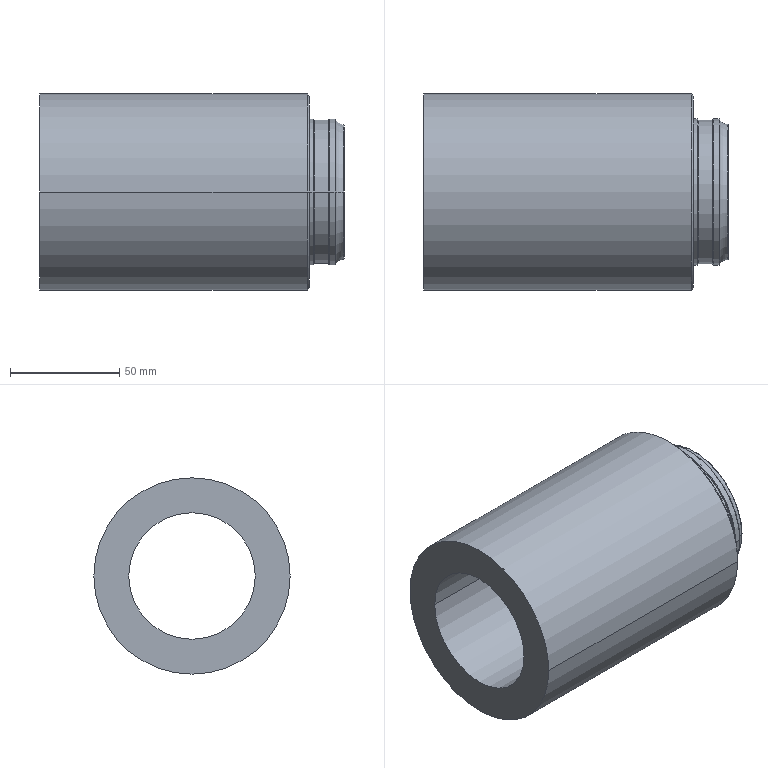Part | SolidWorks | features Revolution 1 | 1 solid | 31 faces | box 139.56 x 90 x 90 mm | volume 471413 mm3 | torus 14 | cylinder 10 | plane 5 | cone 2 | commonest cylinder face diameters 67 x4 58 x2 66 x2 90 x2
STEP:
#1=CARTESIAN_POINT('',(441.026,-31.014,0.));
#2=VERTEX_POINT('',#1);
#3=CARTESIAN_POINT('',(441.026,31.014,0.));
#4=VERTEX_POINT('',#3);
#5=CARTESIAN_POINT('',(441.026,0.,0.));
#6=DIRECTION('',(1.,0.,0.));
#7=DIRECTION('',(0.,1.,0.));
#8=AXIS2_PLACEMENT_3D('',#5,#6,#7);
#9=CIRCLE('',#8,31.014);
#10=EDGE_CURVE('',#2,#4,#9,.T.);
#11=ORIENTED_EDGE('',*,*,#10,.F.);
#12=CARTESIAN_POINT('',(437.44,-33.396,0.));
#13=VERTEX_POINT('',#12);
#14=CARTESIAN_POINT('',(441.503,-35.622,0.));
#15=DIRECTION('',(0.,0.,1.));
#16=DIRECTION('',(0.,-1.,0.));
#17=AXIS2_PLACEMENT_3D('',#14,#15,#16);
#18=CIRCLE('',#17,4.633);
#19=EDGE_CURVE('',#2,#13,#18,.T.);
#20=ORIENTED_EDGE('',*,*,#19,.T.);
#21=CARTESIAN_POINT('',(437.44,33.396,0.));
#22=VERTEX_POINT('',#21);
#23=CARTESIAN_POINT('',(437.44,0.,0.));
#24=DIRECTION('',(1.,0.,0.));
#25=DIRECTION('',(0.,1.,0.));
#26=AXIS2_PLACEMENT_3D('',#23,#24,#25);
#27=CIRCLE('',#26,33.396);
#28=EDGE_CURVE('',#13,#22,#27,.T.);
#29=ORIENTED_EDGE('',*,*,#28,.T.);
#30=CARTESIAN_POINT('',(441.503,35.622,0.));
#31=DIRECTION('',(0.,0.,-1.));
#32=DIRECTION('',(-1.,0.,0.));
#33=AXIS2_PLACEMENT_3D('',#30,#31,#32);
#34=CIRCLE('',#33,4.633);
#35=EDGE_CURVE('',#4,#22,#34,.T.);
#36=ORIENTED_EDGE('',*,*,#35,.F.);
#37=EDGE_LOOP('',(#11,#20,#29,#36));
#38=FACE_OUTER_BOUND('',#37,.T.);
#39=CARTESIAN_POINT('',(441.503,0.,0.));
#40=DIRECTION('',(1.,0.,0.));
#41=DIRECTION('',(0.,1.,0.));
#42=AXIS2_PLACEMENT_3D('',#39,#40,#41);
#43=TOROIDAL_SURFACE('',#42,35.622,4.633);
#44=ADVANCED_FACE('',(#38),#43,.F.);
#45=CARTESIAN_POINT('',(441.026,0.,0.));
#46=DIRECTION('',(1.,0.,0.));
#47=DIRECTION('',(0.,1.,0.));
#48=AXIS2_PLACEMENT_3D('',#45,#46,#47);
#49=CIRCLE('',#48,31.014);
#50=EDGE_CURVE('',#4,#2,#49,.T.);
#51=ORIENTED_EDGE('',*,*,#50,.T.);
#52=CARTESIAN_POINT('',(441.384,-30.616,0.));
#53=VERTEX_POINT('',#52);
#54=CARTESIAN_POINT('',(440.984,-30.616,0.));
#55=DIRECTION('',(0.,0.,1.));
#56=DIRECTION('',(0.,-1.,0.));
#57=AXIS2_PLACEMENT_3D('',#54,#55,#56);
#58=CIRCLE('',#57,0.4);
#59=EDGE_CURVE('',#2,#53,#58,.T.);
#60=ORIENTED_EDGE('',*,*,#59,.T.);
#61=CARTESIAN_POINT('',(441.384,30.616,0.));
#62=VERTEX_POINT('',#61);
#63=CARTESIAN_POINT('',(441.384,0.,0.));
#64=DIRECTION('',(1.,0.,0.));
#65=DIRECTION('',(0.,1.,0.));
#66=AXIS2_PLACEMENT_3D('',#63,#64,#65);
#67=CIRCLE('',#66,30.616);
#68=EDGE_CURVE('',#62,#53,#67,.T.);
#69=ORIENTED_EDGE('',*,*,#68,.F.);
#70=CARTESIAN_POINT('',(440.984,30.616,0.));
#71=DIRECTION('',(0.,0.,-1.));
#72=DIRECTION('',(-1.,0.,0.));
#73=AXIS2_PLACEMENT_3D('',#70,#71,#72);
#74=CIRCLE('',#73,0.4);
#75=EDGE_CURVE('',#4,#62,#74,.T.);
#76=ORIENTED_EDGE('',*,*,#75,.F.);
#77=EDGE_LOOP('',(#51,#60,#69,#76));
#78=FACE_OUTER_BOUND('',#77,.T.);
#79=CARTESIAN_POINT('',(440.984,0.,0.));
#80=DIRECTION('',(1.,0.,0.));
#81=DIRECTION('',(0.,1.,0.));
#82=AXIS2_PLACEMENT_3D('',#79,#80,#81);
#83=TOROIDAL_SURFACE('',#82,30.616,0.4);
#84=ADVANCED_FACE('',(#78),#83,.T.);
#85=CARTESIAN_POINT('',(301.824,-29.,0.));
#86=VERTEX_POINT('',#85);
#87=CARTESIAN_POINT('',(301.824,29.,0.));
#88=VERTEX_POINT('',#87);
#89=CARTESIAN_POINT('',(301.824,0.,0.));
#90=DIRECTION('',(1.,0.,0.));
#91=DIRECTION('',(0.,1.,0.));
#92=AXIS2_PLACEMENT_3D('',#89,#90,#91);
#93=CIRCLE('',#92,29.);
#94=EDGE_CURVE('',#86,#88,#93,.T.);
#95=ORIENTED_EDGE('',*,*,#94,.F.);
#96=CARTESIAN_POINT('',(441.384,-29.,0.));
#97=VERTEX_POINT('',#96);
#98=CARTESIAN_POINT('',(597.174,-29.,0.));
#99=DIRECTION('',(1.,0.,0.));
#100=VECTOR('',#99,1000.);
#101=LINE('',#98,#100);
#102=EDGE_CURVE('',#86,#97,#101,.T.);
#103=ORIENTED_EDGE('',*,*,#102,.T.);
#104=CARTESIAN_POINT('',(441.384,29.,0.));
#105=VERTEX_POINT('',#104);
#106=CARTESIAN_POINT('',(441.384,0.,0.));
#107=DIRECTION('',(1.,0.,0.));
#108=DIRECTION('',(0.,1.,0.));
#109=AXIS2_PLACEMENT_3D('',#106,#107,#108);
#110=CIRCLE('',#109,29.);
#111=EDGE_CURVE('',#97,#105,#110,.T.);
#112=ORIENTED_EDGE('',*,*,#111,.T.);
#113=CARTESIAN_POINT('',(597.174,29.,0.));
#114=DIRECTION('',(1.,0.,0.));
#115=VECTOR('',#114,1000.);
#116=LINE('',#113,#115);
#117=EDGE_CURVE('',#88,#105,#116,.T.);
#118=ORIENTED_EDGE('',*,*,#117,.F.);
#119=EDGE_LOOP('',(#95,#103,#112,#118));
#120=FACE_OUTER_BOUND('',#119,.T.);
#121=CARTESIAN_POINT('',(597.174,0.,0.));
#122=DIRECTION('',(1.,0.,0.));
#123=DIRECTION('',(0.,1.,0.));
#124=AXIS2_PLACEMENT_3D('',#121,#122,#123);
#125=CYLINDRICAL_SURFACE('',#124,29.);
#126=ADVANCED_FACE('',(#120),#125,.F.);
#127=CARTESIAN_POINT('',(301.824,45.,0.));
#128=VERTEX_POINT('',#127);
#129=CARTESIAN_POINT('',(301.824,-45.,0.));
#130=VERTEX_POINT('',#129);
#131=CARTESIAN_POINT('',(301.824,0.,0.));
#132=DIRECTION('',(1.,0.,0.));
#133=DIRECTION('',(0.,1.,0.));
#134=AXIS2_PLACEMENT_3D('',#131,#132,#133);
#135=CIRCLE('',#134,45.);
#136=EDGE_CURVE('',#128,#130,#135,.T.);
#137=ORIENTED_EDGE('',*,*,#136,.T.);
#138=CARTESIAN_POINT('',(424.384,-45.,0.));
#139=VERTEX_POINT('',#138);
#140=CARTESIAN_POINT('',(597.174,-45.,0.));
#141=DIRECTION('',(1.,0.,0.));
#142=VECTOR('',#141,1000.);
#143=LINE('',#140,#142);
#144=EDGE_CURVE('',#130,#139,#143,.T.);
#145=ORIENTED_EDGE('',*,*,#144,.T.);
#146=CARTESIAN_POINT('',(424.384,45.,0.));
#147=VERTEX_POINT('',#146);
#148=CARTESIAN_POINT('',(424.384,0.,0.));
#149=DIRECTION('',(1.,0.,0.));
#150=DIRECTION('',(0.,1.,0.));
#151=AXIS2_PLACEMENT_3D('',#148,#149,#150);
#152=CIRCLE('',#151,45.);
#153=EDGE_CURVE('',#147,#139,#152,.T.);
#154=ORIENTED_EDGE('',*,*,#153,.F.);
#155=CARTESIAN_POINT('',(597.174,45.,0.));
#156=DIRECTION('',(1.,0.,0.));
#157=VECTOR('',#156,1000.);
#158=LINE('',#155,#157);
#159=EDGE_CURVE('',#128,#147,#158,.T.);
#160=ORIENTED_EDGE('',*,*,#159,.F.);
#161=EDGE_LOOP('',(#137,#145,#154,#160));
#162=FACE_OUTER_BOUND('',#161,.T.);
#163=CARTESIAN_POINT('',(597.174,0.,0.));
#164=DIRECTION('',(1.,0.,0.));
#165=DIRECTION('',(0.,1.,0.));
#166=AXIS2_PLACEMENT_3D('',#163,#164,#165);
#167=CYLINDRICAL_SURFACE('',#166,45.);
#168=ADVANCED_FACE('',(#162),#167,.T.);
#169=CARTESIAN_POINT('',(425.384,44.,0.));
#170=VERTEX_POINT('',#169);
#171=CARTESIAN_POINT('',(425.384,-44.,0.));
#172=VERTEX_POINT('',#171);
#173=CARTESIAN_POINT('',(425.384,0.,0.));
#174=DIRECTION('',(1.,0.,0.));
#175=DIRECTION('',(0.,1.,0.));
#176=AXIS2_PLACEMENT_3D('',#173,#174,#175);
#177=CIRCLE('',#176,44.);
#178=EDGE_CURVE('',#170,#172,#177,.T.);
#179=ORIENTED_EDGE('',*,*,#178,.F.);
#180=CARTESIAN_POINT('',(425.384,44.,0.));
#181=DIRECTION('',(-0.7071,0.7071,0.));
#182=VECTOR('',#181,1000.);
#183=LINE('',#180,#182);
#184=EDGE_CURVE('',#170,#147,#183,.T.);
#185=ORIENTED_EDGE('',*,*,#184,.T.);
#186=ORIENTED_EDGE('',*,*,#153,.T.);
#187=CARTESIAN_POINT('',(425.384,-44.,0.));
#188=DIRECTION('',(-0.7071,-0.7071,0.));
#189=VECTOR('',#188,1000.);
#190=LINE('',#187,#189);
#191=EDGE_CURVE('',#172,#139,#190,.T.);
#192=ORIENTED_EDGE('',*,*,#191,.F.);
#193=EDGE_LOOP('',(#179,#185,#186,#192));
#194=FACE_OUTER_BOUND('',#193,.T.);
#195=CARTESIAN_POINT('',(425.384,0.,0.));
#196=DIRECTION('',(-1.,0.,0.));
#197=DIRECTION('',(0.,-1.,0.));
#198=AXIS2_PLACEMENT_3D('',#195,#196,#197);
#199=CONICAL_SURFACE('',#198,44.,0.7854);
#200=ADVANCED_FACE('',(#194),#199,.T.);
#201=CARTESIAN_POINT('',(425.384,33.5,0.));
#202=VERTEX_POINT('',#201);
#203=CARTESIAN_POINT('',(425.384,-33.5,0.));
#204=VERTEX_POINT('',#203);
#205=CARTESIAN_POINT('',(425.384,0.,0.));
#206=DIRECTION('',(1.,0.,0.));
#207=DIRECTION('',(0.,1.,0.));
#208=AXIS2_PLACEMENT_3D('',#205,#206,#207);
#209=CIRCLE('',#208,33.5);
#210=EDGE_CURVE('',#202,#204,#209,.T.);
#211=ORIENTED_EDGE('',*,*,#210,.T.);
#212=CARTESIAN_POINT('',(427.184,-33.5,0.));
#213=VERTEX_POINT('',#212);
#214=CARTESIAN_POINT('',(597.174,-33.5,0.));
#215=DIRECTION('',(1.,0.,0.));
#216=VECTOR('',#215,1000.);
#217=LINE('',#214,#216);
#218=EDGE_CURVE('',#204,#213,#217,.T.);
#219=ORIENTED_EDGE('',*,*,#218,.T.);
#220=CARTESIAN_POINT('',(427.184,33.5,0.));
#221=VERTEX_POINT('',#220);
#222=CARTESIAN_POINT('',(427.184,0.,0.));
#223=DIRECTION('',(1.,0.,0.));
#224=DIRECTION('',(0.,1.,0.));
#225=AXIS2_PLACEMENT_3D('',#222,#223,#224);
#226=CIRCLE('',#225,33.5);
#227=EDGE_CURVE('',#221,#213,#226,.T.);
#228=ORIENTED_EDGE('',*,*,#227,.F.);
#229=CARTESIAN_POINT('',(597.174,33.5,0.));
#230=DIRECTION('',(1.,0.,0.));
#231=VECTOR('',#230,1000.);
#232=LINE('',#229,#231);
#233=EDGE_CURVE('',#202,#221,#232,.T.);
#234=ORIENTED_EDGE('',*,*,#233,.F.);
#235=EDGE_LOOP('',(#211,#219,#228,#234));
#236=FACE_OUTER_BOUND('',#235,.T.);
#237=CARTESIAN_POINT('',(597.174,0.,0.));
#238=DIRECTION('',(1.,0.,0.));
#239=DIRECTION('',(0.,1.,0.));
#240=AXIS2_PLACEMENT_3D('',#237,#238,#239);
#241=CYLINDRICAL_SURFACE('',#240,33.5);
#242=ADVANCED_FACE('',(#236),#241,.T.);
#243=ORIENTED_EDGE('',*,*,#227,.T.);
#244=CARTESIAN_POINT('',(427.384,-33.3,0.));
#245=VERTEX_POINT('',#244);
#246=CARTESIAN_POINT('',(427.184,-33.3,0.));
#247=DIRECTION('',(0.,0.,1.));
#248=DIRECTION('',(0.,-1.,0.));
#249=AXIS2_PLACEMENT_3D('',#246,#247,#248);
#250=CIRCLE('',#249,0.2);
#251=EDGE_CURVE('',#213,#245,#250,.T.);
#252=ORIENTED_EDGE('',*,*,#251,.T.);
#253=CARTESIAN_POINT('',(427.384,33.3,0.));
#254=VERTEX_POINT('',#253);
#255=CARTESIAN_POINT('',(427.384,0.,0.));
#256=DIRECTION('',(1.,0.,0.));
#257=DIRECTION('',(0.,1.,0.));
#258=AXIS2_PLACEMENT_3D('',#255,#256,#257);
#259=CIRCLE('',#258,33.3);
#260=EDGE_CURVE('',#254,#245,#259,.T.);
#261=ORIENTED_EDGE('',*,*,#260,.F.);
#262=CARTESIAN_POINT('',(427.184,33.3,0.));
#263=DIRECTION('',(0.,0.,-1.));
#264=DIRECTION('',(-1.,0.,0.));
#265=AXIS2_PLACEMENT_3D('',#262,#263,#264);
#266=CIRCLE('',#265,0.2);
#267=EDGE_CURVE('',#221,#254,#266,.T.);
#268=ORIENTED_EDGE('',*,*,#267,.F.);
#269=EDGE_LOOP('',(#243,#252,#261,#268));
#270=FACE_OUTER_BOUND('',#269,.T.);
#271=CARTESIAN_POINT('',(427.184,0.,0.));
#272=DIRECTION('',(1.,0.,0.));
#273=DIRECTION('',(0.,1.,0.));
#274=AXIS2_PLACEMENT_3D('',#271,#272,#273);
#275=TOROIDAL_SURFACE('',#274,33.3,0.2);
#276=ADVANCED_FACE('',(#270),#275,.T.);
#277=CARTESIAN_POINT('',(427.584,-33.,0.));
#278=VERTEX_POINT('',#277);
#279=CARTESIAN_POINT('',(427.584,33.,0.));
#280=VERTEX_POINT('',#279);
#281=CARTESIAN_POINT('',(427.584,0.,0.));
#282=DIRECTION('',(1.,0.,0.));
#283=DIRECTION('',(0.,1.,0.));
#284=AXIS2_PLACEMENT_3D('',#281,#282,#283);
#285=CIRCLE('',#284,33.);
#286=EDGE_CURVE('',#278,#280,#285,.T.);
#287=ORIENTED_EDGE('',*,*,#286,.F.);
#288=CARTESIAN_POINT('',(427.384,-33.2,0.));
#289=VERTEX_POINT('',#288);
#290=CARTESIAN_POINT('',(427.584,-33.2,0.));
#291=DIRECTION('',(0.,0.,1.));
#292=DIRECTION('',(0.,-1.,0.));
#293=AXIS2_PLACEMENT_3D('',#290,#291,#292);
#294=CIRCLE('',#293,0.2);
#295=EDGE_CURVE('',#278,#289,#294,.T.);
#296=ORIENTED_EDGE('',*,*,#295,.T.);
#297=CARTESIAN_POINT('',(427.384,33.2,0.));
#298=VERTEX_POINT('',#297);
#299=CARTESIAN_POINT('',(427.384,0.,0.));
#300=DIRECTION('',(1.,0.,0.));
#301=DIRECTION('',(0.,1.,0.));
#302=AXIS2_PLACEMENT_3D('',#299,#300,#301);
#303=CIRCLE('',#302,33.2);
#304=EDGE_CURVE('',#289,#298,#303,.T.);
#305=ORIENTED_EDGE('',*,*,#304,.T.);
#306=CARTESIAN_POINT('',(427.584,33.2,0.));
#307=DIRECTION('',(0.,0.,-1.));
#308=DIRECTION('',(-1.,0.,0.));
#309=AXIS2_PLACEMENT_3D('',#306,#307,#308);
#310=CIRCLE('',#309,0.2);
#311=EDGE_CURVE('',#280,#298,#310,.T.);
#312=ORIENTED_EDGE('',*,*,#311,.F.);
#313=EDGE_LOOP('',(#287,#296,#305,#312));
#314=FACE_OUTER_BOUND('',#313,.T.);
#315=CARTESIAN_POINT('',(427.584,0.,0.));
#316=DIRECTION('',(1.,0.,0.));
#317=DIRECTION('',(0.,1.,0.));
#318=AXIS2_PLACEMENT_3D('',#315,#316,#317);
#319=TOROIDAL_SURFACE('',#318,33.2,0.2);
#320=ADVANCED_FACE('',(#314),#319,.F.);
#321=CARTESIAN_POINT('',(427.584,0.,0.));
#322=DIRECTION('',(1.,0.,0.));
#323=DIRECTION('',(0.,1.,0.));
#324=AXIS2_PLACEMENT_3D('',#321,#322,#323);
#325=CIRCLE('',#324,33.);
#326=EDGE_CURVE('',#280,#278,#325,.T.);
#327=ORIENTED_EDGE('',*,*,#326,.T.);
#328=CARTESIAN_POINT('',(434.184,-33.,0.));
#329=VERTEX_POINT('',#328);
#330=CARTESIAN_POINT('',(597.174,-33.,0.));
#331=DIRECTION('',(1.,0.,0.));
#332=VECTOR('',#331,1000.);
#333=LINE('',#330,#332);
#334=EDGE_CURVE('',#278,#329,#333,.T.);
#335=ORIENTED_EDGE('',*,*,#334,.T.);
#336=CARTESIAN_POINT('',(434.184,33.,0.));
#337=VERTEX_POINT('',#336);
#338=CARTESIAN_POINT('',(434.184,0.,0.));
#339=DIRECTION('',(1.,0.,0.));
#340=DIRECTION('',(0.,1.,0.));
#341=AXIS2_PLACEMENT_3D('',#338,#339,#340);
#342=CIRCLE('',#341,33.);
#343=EDGE_CURVE('',#337,#329,#342,.T.);
#344=ORIENTED_EDGE('',*,*,#343,.F.);
#345=CARTESIAN_POINT('',(597.174,33.,0.));
#346=DIRECTION('',(1.,0.,0.));
#347=VECTOR('',#346,1000.);
#348=LINE('',#345,#347);
#349=EDGE_CURVE('',#280,#337,#348,.T.);
#350=ORIENTED_EDGE('',*,*,#349,.F.);
#351=EDGE_LOOP('',(#327,#335,#344,#350));
#352=FACE_OUTER_BOUND('',#351,.T.);
#353=CARTESIAN_POINT('',(597.174,0.,0.));
#354=DIRECTION('',(1.,0.,0.));
#355=DIRECTION('',(0.,1.,0.));
#356=AXIS2_PLACEMENT_3D('',#353,#354,#355);
#357=CYLINDRICAL_SURFACE('',#356,33.);
#358=ADVANCED_FACE('',(#352),#357,.T.);
#359=CARTESIAN_POINT('',(434.384,-33.2,0.));
#360=VERTEX_POINT('',#359);
#361=CARTESIAN_POINT('',(434.384,33.2,0.));
#362=VERTEX_POINT('',#361);
#363=CARTESIAN_POINT('',(434.384,0.,0.));
#364=DIRECTION('',(1.,0.,0.));
#365=DIRECTION('',(0.,1.,0.));
#366=AXIS2_PLACEMENT_3D('',#363,#364,#365);
#367=CIRCLE('',#366,33.2);
#368=EDGE_CURVE('',#360,#362,#367,.T.);
#369=ORIENTED_EDGE('',*,*,#368,.F.);
#370=CARTESIAN_POINT('',(434.184,-33.2,0.));
#371=DIRECTION('',(0.,0.,1.));
#372=DIRECTION('',(0.,-1.,0.));
#373=AXIS2_PLACEMENT_3D('',#370,#371,#372);
#374=CIRCLE('',#373,0.2);
#375=EDGE_CURVE('',#360,#329,#374,.T.);
#376=ORIENTED_EDGE('',*,*,#375,.T.);
#377=CARTESIAN_POINT('',(434.184,0.,0.));
#378=DIRECTION('',(1.,0.,0.));
#379=DIRECTION('',(0.,1.,0.));
#380=AXIS2_PLACEMENT_3D('',#377,#378,#379);
#381=CIRCLE('',#380,33.);
#382=EDGE_CURVE('',#329,#337,#381,.T.);
#383=ORIENTED_EDGE('',*,*,#382,.T.);
#384=CARTESIAN_POINT('',(434.184,33.2,0.));
#385=DIRECTION('',(0.,0.,-1.));
#386=DIRECTION('',(-1.,0.,0.));
#387=AXIS2_PLACEMENT_3D('',#384,#385,#386);
#388=CIRCLE('',#387,0.2);
#389=EDGE_CURVE('',#362,#337,#388,.T.);
#390=ORIENTED_EDGE('',*,*,#389,.F.);
#391=EDGE_LOOP('',(#369,#376,#383,#390));
#392=FACE_OUTER_BOUND('',#391,.T.);
#393=CARTESIAN_POINT('',(434.184,0.,0.));
#394=DIRECTION('',(1.,0.,0.));
#395=DIRECTION('',(0.,1.,0.));
#396=AXIS2_PLACEMENT_3D('',#393,#394,#395);
#397=TOROIDAL_SURFACE('',#396,33.2,0.2);
#398=ADVANCED_FACE('',(#392),#397,.F.);
#399=CARTESIAN_POINT('',(434.384,33.3,0.));
#400=VERTEX_POINT('',#399);
#401=CARTESIAN_POINT('',(434.384,-33.3,0.));
#402=VERTEX_POINT('',#401);
#403=CARTESIAN_POINT('',(434.384,0.,0.));
#404=DIRECTION('',(1.,0.,0.));
#405=DIRECTION('',(0.,1.,0.));
#406=AXIS2_PLACEMENT_3D('',#403,#404,#405);
#407=CIRCLE('',#406,33.3);
#408=EDGE_CURVE('',#400,#402,#407,.T.);
#409=ORIENTED_EDGE('',*,*,#408,.T.);
#410=CARTESIAN_POINT('',(434.584,-33.5,0.));
#411=VERTEX_POINT('',#410);
#412=CARTESIAN_POINT('',(434.584,-33.3,0.));
#413=DIRECTION('',(0.,0.,1.));
#414=DIRECTION('',(0.,-1.,0.));
#415=AXIS2_PLACEMENT_3D('',#412,#413,#414);
#416=CIRCLE('',#415,0.2);
#417=EDGE_CURVE('',#402,#411,#416,.T.);
#418=ORIENTED_EDGE('',*,*,#417,.T.);
#419=CARTESIAN_POINT('',(434.584,33.5,0.));
#420=VERTEX_POINT('',#419);
#421=CARTESIAN_POINT('',(434.584,0.,0.));
#422=DIRECTION('',(1.,0.,0.));
#423=DIRECTION('',(0.,1.,0.));
#424=AXIS2_PLACEMENT_3D('',#421,#422,#423);
#425=CIRCLE('',#424,33.5);
#426=EDGE_CURVE('',#420,#411,#425,.T.);
#427=ORIENTED_EDGE('',*,*,#426,.F.);
#428=CARTESIAN_POINT('',(434.584,33.3,0.));
#429=DIRECTION('',(0.,0.,-1.));
#430=DIRECTION('',(-1.,0.,0.));
#431=AXIS2_PLACEMENT_3D('',#428,#429,#430);
#432=CIRCLE('',#431,0.2);
#433=EDGE_CURVE('',#400,#420,#432,.T.);
#434=ORIENTED_EDGE('',*,*,#433,.F.);
#435=EDGE_LOOP('',(#409,#418,#427,#434));
#436=FACE_OUTER_BOUND('',#435,.T.);
#437=CARTESIAN_POINT('',(434.584,0.,0.));
#438=DIRECTION('',(1.,0.,0.));
#439=DIRECTION('',(0.,1.,0.));
#440=AXIS2_PLACEMENT_3D('',#437,#438,#439);
#441=TOROIDAL_SURFACE('',#440,33.3,0.2);
#442=ADVANCED_FACE('',(#436),#441,.T.);
#443=ORIENTED_EDGE('',*,*,#426,.T.);
#444=CARTESIAN_POINT('',(437.264,-33.5,0.));
#445=VERTEX_POINT('',#444);
#446=CARTESIAN_POINT('',(597.174,-33.5,0.));
#447=DIRECTION('',(1.,0.,0.));
#448=VECTOR('',#447,1000.);
#449=LINE('',#446,#448);
#450=EDGE_CURVE('',#411,#445,#449,.T.);
#451=ORIENTED_EDGE('',*,*,#450,.T.);
#452=CARTESIAN_POINT('',(437.264,33.5,0.));
#453=VERTEX_POINT('',#452);
#454=CARTESIAN_POINT('',(437.264,0.,0.));
#455=DIRECTION('',(1.,0.,0.));
#456=DIRECTION('',(0.,1.,0.));
#457=AXIS2_PLACEMENT_3D('',#454,#455,#456);
#458=CIRCLE('',#457,33.5);
#459=EDGE_CURVE('',#453,#445,#458,.T.);
#460=ORIENTED_EDGE('',*,*,#459,.F.);
#461=CARTESIAN_POINT('',(597.174,33.5,0.));
#462=DIRECTION('',(1.,0.,0.));
#463=VECTOR('',#462,1000.);
#464=LINE('',#461,#463);
#465=EDGE_CURVE('',#420,#453,#464,.T.);
#466=ORIENTED_EDGE('',*,*,#465,.F.);
#467=EDGE_LOOP('',(#443,#451,#460,#466));
#468=FACE_OUTER_BOUND('',#467,.T.);
#469=CARTESIAN_POINT('',(597.174,0.,0.));
#470=DIRECTION('',(1.,0.,0.));
#471=DIRECTION('',(0.,1.,0.));
#472=AXIS2_PLACEMENT_3D('',#469,#470,#471);
#473=CYLINDRICAL_SURFACE('',#472,33.5);
#474=ADVANCED_FACE('',(#468),#473,.T.);
#475=ORIENTED_EDGE('',*,*,#459,.T.);
#476=CARTESIAN_POINT('',(437.264,-33.3,0.));
#477=DIRECTION('',(0.,0.,1.));
#478=DIRECTION('',(0.,-1.,0.));
#479=AXIS2_PLACEMENT_3D('',#476,#477,#478);
#480=CIRCLE('',#479,0.2);
#481=EDGE_CURVE('',#445,#13,#480,.T.);
#482=ORIENTED_EDGE('',*,*,#481,.T.);
#483=CARTESIAN_POINT('',(437.44,0.,0.));
#484=DIRECTION('',(1.,0.,0.));
#485=DIRECTION('',(0.,1.,0.));
#486=AXIS2_PLACEMENT_3D('',#483,#484,#485);
#487=CIRCLE('',#486,33.396);
#488=EDGE_CURVE('',#22,#13,#487,.T.);
#489=ORIENTED_EDGE('',*,*,#488,.F.);
#490=CARTESIAN_POINT('',(437.264,33.3,0.));
#491=DIRECTION('',(0.,0.,-1.));
#492=DIRECTION('',(-1.,0.,0.));
#493=AXIS2_PLACEMENT_3D('',#490,#491,#492);
#494=CIRCLE('',#493,0.2);
#495=EDGE_CURVE('',#453,#22,#494,.T.);
#496=ORIENTED_EDGE('',*,*,#495,.F.);
#497=EDGE_LOOP('',(#475,#482,#489,#496));
#498=FACE_OUTER_BOUND('',#497,.T.);
#499=CARTESIAN_POINT('',(437.264,0.,0.));
#500=DIRECTION('',(1.,0.,0.));
#501=DIRECTION('',(0.,1.,0.));
#502=AXIS2_PLACEMENT_3D('',#499,#500,#501);
#503=TOROIDAL_SURFACE('',#502,33.3,0.2);
#504=ADVANCED_FACE('',(#498),#503,.T.);
#505=ORIENTED_EDGE('',*,*,#481,.F.);
#506=CARTESIAN_POINT('',(437.264,0.,0.));
#507=DIRECTION('',(1.,0.,0.));
#508=DIRECTION('',(0.,1.,0.));
#509=AXIS2_PLACEMENT_3D('',#506,#507,#508);
#510=CIRCLE('',#509,33.5);
#511=EDGE_CURVE('',#445,#453,#510,.T.);
#512=ORIENTED_EDGE('',*,*,#511,.T.);
#513=ORIENTED_EDGE('',*,*,#495,.T.);
#514=ORIENTED_EDGE('',*,*,#28,.F.);
#515=EDGE_LOOP('',(#505,#512,#513,#514));
#516=FACE_OUTER_BOUND('',#515,.T.);
#517=CARTESIAN_POINT('',(437.264,0.,0.));
#518=DIRECTION('',(1.,0.,0.));
#519=DIRECTION('',(0.,1.,0.));
#520=AXIS2_PLACEMENT_3D('',#517,#518,#519);
#521=TOROIDAL_SURFACE('',#520,33.3,0.2);
#522=ADVANCED_FACE('',(#516),#521,.T.);
#523=ORIENTED_EDGE('',*,*,#450,.F.);
#524=CARTESIAN_POINT('',(434.584,0.,0.));
#525=DIRECTION('',(1.,0.,0.));
#526=DIRECTION('',(0.,1.,0.));
#527=AXIS2_PLACEMENT_3D('',#524,#525,#526);
#528=CIRCLE('',#527,33.5);
#529=EDGE_CURVE('',#411,#420,#528,.T.);
#530=ORIENTED_EDGE('',*,*,#529,.T.);
#531=ORIENTED_EDGE('',*,*,#465,.T.);
#532=ORIENTED_EDGE('',*,*,#511,.F.);
#533=EDGE_LOOP('',(#523,#530,#531,#532));
#534=FACE_OUTER_BOUND('',#533,.T.);
#535=CARTESIAN_POINT('',(597.174,0.,0.));
#536=DIRECTION('',(1.,0.,0.));
#537=DIRECTION('',(0.,1.,0.));
#538=AXIS2_PLACEMENT_3D('',#535,#536,#537);
#539=CYLINDRICAL_SURFACE('',#538,33.5);
#540=ADVANCED_FACE('',(#534),#539,.T.);
#541=ORIENTED_EDGE('',*,*,#417,.F.);
#542=CARTESIAN_POINT('',(434.384,0.,0.));
#543=DIRECTION('',(1.,0.,0.));
#544=DIRECTION('',(0.,1.,0.));
#545=AXIS2_PLACEMENT_3D('',#542,#543,#544);
#546=CIRCLE('',#545,33.3);
#547=EDGE_CURVE('',#402,#400,#546,.T.);
#548=ORIENTED_EDGE('',*,*,#547,.T.);
#549=ORIENTED_EDGE('',*,*,#433,.T.);
#550=ORIENTED_EDGE('',*,*,#529,.F.);
#551=EDGE_LOOP('',(#541,#548,#549,#550));
#552=FACE_OUTER_BOUND('',#551,.T.);
#553=CARTESIAN_POINT('',(434.584,0.,0.));
#554=DIRECTION('',(1.,0.,0.));
#555=DIRECTION('',(0.,1.,0.));
#556=AXIS2_PLACEMENT_3D('',#553,#554,#555);
#557=TOROIDAL_SURFACE('',#556,33.3,0.2);
#558=ADVANCED_FACE('',(#552),#557,.T.);
#559=CARTESIAN_POINT('',(434.384,0.,0.));
#560=DIRECTION('',(1.,0.,0.));
#561=DIRECTION('',(0.,1.,0.));
#562=AXIS2_PLACEMENT_3D('',#559,#560,#561);
#563=CIRCLE('',#562,33.2);
#564=EDGE_CURVE('',#362,#360,#563,.T.);
#565=ORIENTED_EDGE('',*,*,#564,.T.);
#566=ORIENTED_EDGE('',*,*,#368,.T.);
#567=EDGE_LOOP('',(#565,#566));
#568=FACE_BOUND('',#567,.T.);
#569=ORIENTED_EDGE('',*,*,#408,.F.);
#570=ORIENTED_EDGE('',*,*,#547,.F.);
#571=EDGE_LOOP('',(#569,#570));
#572=FACE_OUTER_BOUND('',#571,.T.);
#573=CARTESIAN_POINT('',(434.384,33.3,0.));
#574=DIRECTION('',(-1.,0.,0.));
#575=DIRECTION('',(0.,-1.,0.));
#576=AXIS2_PLACEMENT_3D('',#573,#574,#575);
#577=PLANE('',#576);
#578=ADVANCED_FACE('',(#568,#572),#577,.T.);
#579=ORIENTED_EDGE('',*,*,#375,.F.);
#580=ORIENTED_EDGE('',*,*,#564,.F.);
#581=ORIENTED_EDGE('',*,*,#389,.T.);
#582=ORIENTED_EDGE('',*,*,#343,.T.);
#583=EDGE_LOOP('',(#579,#580,#581,#582));
#584=FACE_OUTER_BOUND('',#583,.T.);
#585=CARTESIAN_POINT('',(434.184,0.,0.));
#586=DIRECTION('',(1.,0.,0.));
#587=DIRECTION('',(0.,1.,0.));
#588=AXIS2_PLACEMENT_3D('',#585,#586,#587);
#589=TOROIDAL_SURFACE('',#588,33.2,0.2);
#590=ADVANCED_FACE('',(#584),#589,.F.);
#591=ORIENTED_EDGE('',*,*,#334,.F.);
#592=ORIENTED_EDGE('',*,*,#286,.T.);
#593=ORIENTED_EDGE('',*,*,#349,.T.);
#594=ORIENTED_EDGE('',*,*,#382,.F.);
#595=EDGE_LOOP('',(#591,#592,#593,#594));
#596=FACE_OUTER_BOUND('',#595,.T.);
#597=CARTESIAN_POINT('',(597.174,0.,0.));
#598=DIRECTION('',(1.,0.,0.));
#599=DIRECTION('',(0.,1.,0.));
#600=AXIS2_PLACEMENT_3D('',#597,#598,#599);
#601=CYLINDRICAL_SURFACE('',#600,33.);
#602=ADVANCED_FACE('',(#596),#601,.T.);
#603=ORIENTED_EDGE('',*,*,#295,.F.);
#604=ORIENTED_EDGE('',*,*,#326,.F.);
#605=ORIENTED_EDGE('',*,*,#311,.T.);
#606=CARTESIAN_POINT('',(427.384,0.,0.));
#607=DIRECTION('',(1.,0.,0.));
#608=DIRECTION('',(0.,1.,0.));
#609=AXIS2_PLACEMENT_3D('',#606,#607,#608);
#610=CIRCLE('',#609,33.2);
#611=EDGE_CURVE('',#298,#289,#610,.T.);
#612=ORIENTED_EDGE('',*,*,#611,.T.);
#613=EDGE_LOOP('',(#603,#604,#605,#612));
#614=FACE_OUTER_BOUND('',#613,.T.);
#615=CARTESIAN_POINT('',(427.584,0.,0.));
#616=DIRECTION('',(1.,0.,0.));
#617=DIRECTION('',(0.,1.,0.));
#618=AXIS2_PLACEMENT_3D('',#615,#616,#617);
#619=TOROIDAL_SURFACE('',#618,33.2,0.2);
#620=ADVANCED_FACE('',(#614),#619,.F.);
#621=ORIENTED_EDGE('',*,*,#260,.T.);
#622=CARTESIAN_POINT('',(427.384,0.,0.));
#623=DIRECTION('',(1.,0.,0.));
#624=DIRECTION('',(0.,1.,0.));
#625=AXIS2_PLACEMENT_3D('',#622,#623,#624);
#626=CIRCLE('',#625,33.3);
#627=EDGE_CURVE('',#245,#254,#626,.T.);
#628=ORIENTED_EDGE('',*,*,#627,.T.);
#629=EDGE_LOOP('',(#621,#628));
#630=FACE_OUTER_BOUND('',#629,.T.);
#631=ORIENTED_EDGE('',*,*,#611,.F.);
#632=ORIENTED_EDGE('',*,*,#304,.F.);
#633=EDGE_LOOP('',(#631,#632));
#634=FACE_BOUND('',#633,.T.);
#635=CARTESIAN_POINT('',(427.384,33.3,0.));
#636=DIRECTION('',(1.,0.,0.));
#637=DIRECTION('',(0.,1.,0.));
#638=AXIS2_PLACEMENT_3D('',#635,#636,#637);
#639=PLANE('',#638);
#640=ADVANCED_FACE('',(#630,#634),#639,.T.);
#641=ORIENTED_EDGE('',*,*,#251,.F.);
#642=CARTESIAN_POINT('',(427.184,0.,0.));
#643=DIRECTION('',(1.,0.,0.));
#644=DIRECTION('',(0.,1.,0.));
#645=AXIS2_PLACEMENT_3D('',#642,#643,#644);
#646=CIRCLE('',#645,33.5);
#647=EDGE_CURVE('',#213,#221,#646,.T.);
#648=ORIENTED_EDGE('',*,*,#647,.T.);
#649=ORIENTED_EDGE('',*,*,#267,.T.);
#650=ORIENTED_EDGE('',*,*,#627,.F.);
#651=EDGE_LOOP('',(#641,#648,#649,#650));
#652=FACE_OUTER_BOUND('',#651,.T.);
#653=CARTESIAN_POINT('',(427.184,0.,0.));
#654=DIRECTION('',(1.,0.,0.));
#655=DIRECTION('',(0.,1.,0.));
#656=AXIS2_PLACEMENT_3D('',#653,#654,#655);
#657=TOROIDAL_SURFACE('',#656,33.3,0.2);
#658=ADVANCED_FACE('',(#652),#657,.T.);
#659=ORIENTED_EDGE('',*,*,#218,.F.);
#660=CARTESIAN_POINT('',(425.384,0.,0.));
#661=DIRECTION('',(1.,0.,0.));
#662=DIRECTION('',(0.,1.,0.));
#663=AXIS2_PLACEMENT_3D('',#660,#661,#662);
#664=CIRCLE('',#663,33.5);
#665=EDGE_CURVE('',#204,#202,#664,.T.);
#666=ORIENTED_EDGE('',*,*,#665,.T.);
#667=ORIENTED_EDGE('',*,*,#233,.T.);
#668=ORIENTED_EDGE('',*,*,#647,.F.);
#669=EDGE_LOOP('',(#659,#666,#667,#668));
#670=FACE_OUTER_BOUND('',#669,.T.);
#671=CARTESIAN_POINT('',(597.174,0.,0.));
#672=DIRECTION('',(1.,0.,0.));
#673=DIRECTION('',(0.,1.,0.));
#674=AXIS2_PLACEMENT_3D('',#671,#672,#673);
#675=CYLINDRICAL_SURFACE('',#674,33.5);
#676=ADVANCED_FACE('',(#670),#675,.T.);
#677=CARTESIAN_POINT('',(425.384,0.,0.));
#678=DIRECTION('',(1.,0.,0.));
#679=DIRECTION('',(0.,1.,0.));
#680=AXIS2_PLACEMENT_3D('',#677,#678,#679);
#681=CIRCLE('',#680,44.);
#682=EDGE_CURVE('',#172,#170,#681,.T.);
#683=ORIENTED_EDGE('',*,*,#682,.T.);
#684=ORIENTED_EDGE('',*,*,#178,.T.);
#685=EDGE_LOOP('',(#683,#684));
#686=FACE_OUTER_BOUND('',#685,.T.);
#687=ORIENTED_EDGE('',*,*,#210,.F.);
#688=ORIENTED_EDGE('',*,*,#665,.F.);
#689=EDGE_LOOP('',(#687,#688));
#690=FACE_BOUND('',#689,.T.);
#691=CARTESIAN_POINT('',(425.384,44.,0.));
#692=DIRECTION('',(1.,0.,0.));
#693=DIRECTION('',(0.,1.,0.));
#694=AXIS2_PLACEMENT_3D('',#691,#692,#693);
#695=PLANE('',#694);
#696=ADVANCED_FACE('',(#686,#690),#695,.T.);
#697=ORIENTED_EDGE('',*,*,#184,.F.);
#698=ORIENTED_EDGE('',*,*,#682,.F.);
#699=ORIENTED_EDGE('',*,*,#191,.T.);
#700=CARTESIAN_POINT('',(424.384,0.,0.));
#701=DIRECTION('',(1.,0.,0.));
#702=DIRECTION('',(0.,1.,0.));
#703=AXIS2_PLACEMENT_3D('',#700,#701,#702);
#704=CIRCLE('',#703,45.);
#705=EDGE_CURVE('',#139,#147,#704,.T.);
#706=ORIENTED_EDGE('',*,*,#705,.T.);
#707=EDGE_LOOP('',(#697,#698,#699,#706));
#708=FACE_OUTER_BOUND('',#707,.T.);
#709=CARTESIAN_POINT('',(425.384,0.,0.));
#710=DIRECTION('',(-1.,0.,0.));
#711=DIRECTION('',(0.,-1.,0.));
#712=AXIS2_PLACEMENT_3D('',#709,#710,#711);
#713=CONICAL_SURFACE('',#712,44.,0.7854);
#714=ADVANCED_FACE('',(#708),#713,.T.);
#715=ORIENTED_EDGE('',*,*,#144,.F.);
#716=CARTESIAN_POINT('',(301.824,0.,0.));
#717=DIRECTION('',(1.,0.,0.));
#718=DIRECTION('',(0.,1.,0.));
#719=AXIS2_PLACEMENT_3D('',#716,#717,#718);
#720=CIRCLE('',#719,45.);
#721=EDGE_CURVE('',#130,#128,#720,.T.);
#722=ORIENTED_EDGE('',*,*,#721,.T.);
#723=ORIENTED_EDGE('',*,*,#159,.T.);
#724=ORIENTED_EDGE('',*,*,#705,.F.);
#725=EDGE_LOOP('',(#715,#722,#723,#724));
#726=FACE_OUTER_BOUND('',#725,.T.);
#727=CARTESIAN_POINT('',(597.174,0.,0.));
#728=DIRECTION('',(1.,0.,0.));
#729=DIRECTION('',(0.,1.,0.));
#730=AXIS2_PLACEMENT_3D('',#727,#728,#729);
#731=CYLINDRICAL_SURFACE('',#730,45.);
#732=ADVANCED_FACE('',(#726),#731,.T.);
#733=CARTESIAN_POINT('',(301.824,0.,0.));
#734=DIRECTION('',(1.,0.,0.));
#735=DIRECTION('',(0.,1.,0.));
#736=AXIS2_PLACEMENT_3D('',#733,#734,#735);
#737=CIRCLE('',#736,29.);
#738=EDGE_CURVE('',#88,#86,#737,.T.);
#739=ORIENTED_EDGE('',*,*,#738,.T.);
#740=ORIENTED_EDGE('',*,*,#94,.T.);
#741=EDGE_LOOP('',(#739,#740));
#742=FACE_BOUND('',#741,.T.);
#743=ORIENTED_EDGE('',*,*,#136,.F.);
#744=ORIENTED_EDGE('',*,*,#721,.F.);
#745=EDGE_LOOP('',(#743,#744));
#746=FACE_OUTER_BOUND('',#745,.T.);
#747=CARTESIAN_POINT('',(301.824,45.,0.));
#748=DIRECTION('',(-1.,0.,0.));
#749=DIRECTION('',(0.,-1.,0.));
#750=AXIS2_PLACEMENT_3D('',#747,#748,#749);
#751=PLANE('',#750);
#752=ADVANCED_FACE('',(#742,#746),#751,.T.);
#753=ORIENTED_EDGE('',*,*,#102,.F.);
#754=ORIENTED_EDGE('',*,*,#738,.F.);
#755=ORIENTED_EDGE('',*,*,#117,.T.);
#756=CARTESIAN_POINT('',(441.384,0.,0.));
#757=DIRECTION('',(1.,0.,0.));
#758=DIRECTION('',(0.,1.,0.));
#759=AXIS2_PLACEMENT_3D('',#756,#757,#758);
#760=CIRCLE('',#759,29.);
#761=EDGE_CURVE('',#105,#97,#760,.T.);
#762=ORIENTED_EDGE('',*,*,#761,.T.);
#763=EDGE_LOOP('',(#753,#754,#755,#762));
#764=FACE_OUTER_BOUND('',#763,.T.);
#765=CARTESIAN_POINT('',(597.174,0.,0.));
#766=DIRECTION('',(1.,0.,0.));
#767=DIRECTION('',(0.,1.,0.));
#768=AXIS2_PLACEMENT_3D('',#765,#766,#767);
#769=CYLINDRICAL_SURFACE('',#768,29.);
#770=ADVANCED_FACE('',(#764),#769,.F.);
#771=ORIENTED_EDGE('',*,*,#68,.T.);
#772=CARTESIAN_POINT('',(441.384,0.,0.));
#773=DIRECTION('',(1.,0.,0.));
#774=DIRECTION('',(0.,1.,0.));
#775=AXIS2_PLACEMENT_3D('',#772,#773,#774);
#776=CIRCLE('',#775,30.616);
#777=EDGE_CURVE('',#53,#62,#776,.T.);
#778=ORIENTED_EDGE('',*,*,#777,.T.);
#779=EDGE_LOOP('',(#771,#778));
#780=FACE_OUTER_BOUND('',#779,.T.);
#781=ORIENTED_EDGE('',*,*,#761,.F.);
#782=ORIENTED_EDGE('',*,*,#111,.F.);
#783=EDGE_LOOP('',(#781,#782));
#784=FACE_BOUND('',#783,.T.);
#785=CARTESIAN_POINT('',(441.384,30.616,0.));
#786=DIRECTION('',(1.,0.,0.));
#787=DIRECTION('',(0.,1.,0.));
#788=AXIS2_PLACEMENT_3D('',#785,#786,#787);
#789=PLANE('',#788);
#790=ADVANCED_FACE('',(#780,#784),#789,.T.);
#791=ORIENTED_EDGE('',*,*,#59,.F.);
#792=ORIENTED_EDGE('',*,*,#10,.T.);
#793=ORIENTED_EDGE('',*,*,#75,.T.);
#794=ORIENTED_EDGE('',*,*,#777,.F.);
#795=EDGE_LOOP('',(#791,#792,#793,#794));
#796=FACE_OUTER_BOUND('',#795,.T.);
#797=CARTESIAN_POINT('',(440.984,0.,0.));
#798=DIRECTION('',(1.,0.,0.));
#799=DIRECTION('',(0.,1.,0.));
#800=AXIS2_PLACEMENT_3D('',#797,#798,#799);
#801=TOROIDAL_SURFACE('',#800,30.616,0.4);
#802=ADVANCED_FACE('',(#796),#801,.T.);
#803=ORIENTED_EDGE('',*,*,#19,.F.);
#804=ORIENTED_EDGE('',*,*,#50,.F.);
#805=ORIENTED_EDGE('',*,*,#35,.T.);
#806=ORIENTED_EDGE('',*,*,#488,.T.);
#807=EDGE_LOOP('',(#803,#804,#805,#806));
#808=FACE_OUTER_BOUND('',#807,.T.);
#809=CARTESIAN_POINT('',(441.503,0.,0.));
#810=DIRECTION('',(1.,0.,0.));
#811=DIRECTION('',(0.,1.,0.));
#812=AXIS2_PLACEMENT_3D('',#809,#810,#811);
#813=TOROIDAL_SURFACE('',#812,35.622,4.633);
#814=ADVANCED_FACE('',(#808),#813,.F.);
#815=CLOSED_SHELL('',(#44,#84,#126,#168,#200,#242,#276,#320,#358,#398,#442,#474,#504,#522,#540,#558,#578,#590,#602,#620,#640,#658,#676,#696,#714,#732,#752,#770,#790,#802,#814));
#816=MANIFOLD_SOLID_BREP('',#815);
#817=CARTESIAN_POINT('',(0.,0.,0.));
#818=DIRECTION('',(0.,0.,1.));
#819=DIRECTION('',(1.,0.,0.));
#820=AXIS2_PLACEMENT_3D('',#817,#818,#819);
#821=(LENGTH_UNIT()NAMED_UNIT(*)SI_UNIT(.MILLI.,.METRE.));
#822=UNCERTAINTY_MEASURE_WITH_UNIT(LENGTH_MEASURE(0.00001),#821,'','');
#823=(NAMED_UNIT(*)PLANE_ANGLE_UNIT()SI_UNIT($,.RADIAN.));
#824=(NAMED_UNIT(*)SI_UNIT($,.STERADIAN.)SOLID_ANGLE_UNIT());
#825=(GEOMETRIC_REPRESENTATION_CONTEXT(3)GLOBAL_UNCERTAINTY_ASSIGNED_CONTEXT((#822))GLOBAL_UNIT_ASSIGNED_CONTEXT((#821,#823,#824))REPRESENTATION_CONTEXT('',''));
#826=ADVANCED_BREP_SHAPE_REPRESENTATION('',(#816,#820),#825);